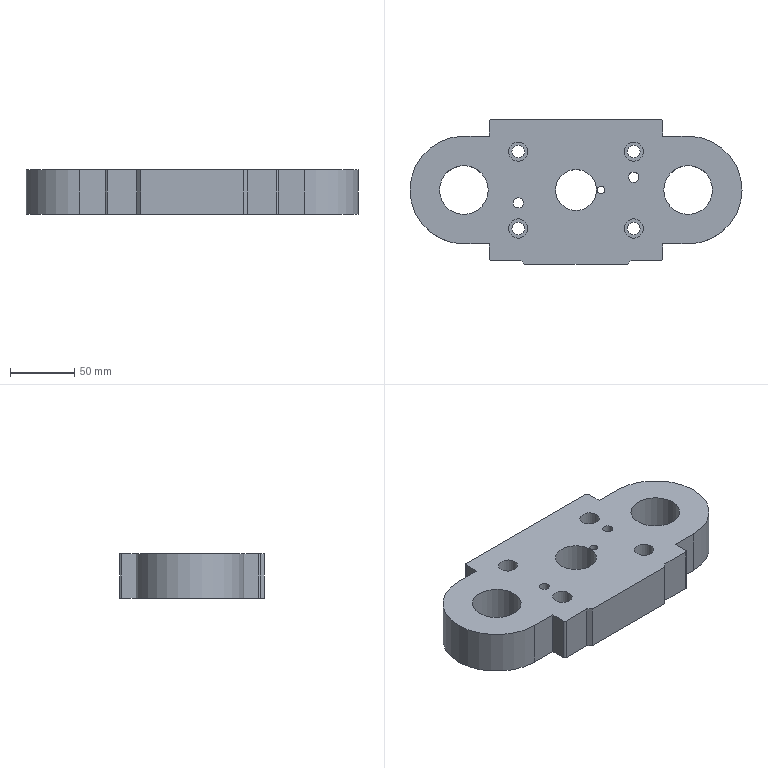Part | NX | features EXTRUDE 3, DATUM_CSYS 2, SKETCH 1 | 1 solid | 42 faces | box 259 x 113 x 35 mm | volume 709332 mm3 | cylinder 21 | plane 21 | commonest cylinder face diameters 3 x4 10 x4 15 x4 8 x2 38 x2 84 x2
STEP:
#1=CARTESIAN_POINT('',(22.5,0.,35.));
#2=VERTEX_POINT('',#1);
#3=CARTESIAN_POINT('',(19.5,0.,35.));
#4=DIRECTION('',(0.,0.,1.));
#5=DIRECTION('',(1.,0.,0.));
#6=AXIS2_PLACEMENT_3D('',#3,#4,#5);
#7=CIRCLE('',#6,3.);
#8=EDGE_CURVE('',#2,#2,#7,.T.);
#9=ORIENTED_EDGE('',*,*,#8,.T.);
#10=EDGE_LOOP('',(#9));
#11=FACE_BOUND('',#10,.T.);
#12=CARTESIAN_POINT('',(20.295,2.893,5.));
#13=VERTEX_POINT('',#12);
#14=CARTESIAN_POINT('',(20.295,-2.893,5.));
#15=VERTEX_POINT('',#14);
#16=CARTESIAN_POINT('',(19.5,0.,5.));
#17=DIRECTION('',(0.,0.,1.));
#18=DIRECTION('',(1.,0.,0.));
#19=AXIS2_PLACEMENT_3D('',#16,#17,#18);
#20=CIRCLE('',#19,3.);
#21=EDGE_CURVE('',#13,#15,#20,.T.);
#22=ORIENTED_EDGE('',*,*,#21,.F.);
#23=CARTESIAN_POINT('',(20.295,2.893,0.));
#24=VERTEX_POINT('',#23);
#25=CARTESIAN_POINT('',(20.295,2.893,2.5));
#26=DIRECTION('',(0.,0.,-1.));
#27=VECTOR('',#26,1000.);
#28=LINE('',#25,#27);
#29=EDGE_CURVE('',#13,#24,#28,.T.);
#30=ORIENTED_EDGE('',*,*,#29,.T.);
#31=CARTESIAN_POINT('',(20.295,-2.893,0.));
#32=VERTEX_POINT('',#31);
#33=CARTESIAN_POINT('',(19.5,0.,0.));
#34=DIRECTION('',(0.,0.,1.));
#35=DIRECTION('',(1.,0.,0.));
#36=AXIS2_PLACEMENT_3D('',#33,#34,#35);
#37=CIRCLE('',#36,3.);
#38=EDGE_CURVE('',#32,#24,#37,.T.);
#39=ORIENTED_EDGE('',*,*,#38,.F.);
#40=CARTESIAN_POINT('',(20.295,-2.893,2.5));
#41=DIRECTION('',(0.,0.,-1.));
#42=VECTOR('',#41,1000.);
#43=LINE('',#40,#42);
#44=EDGE_CURVE('',#32,#15,#43,.F.);
#45=ORIENTED_EDGE('',*,*,#44,.T.);
#46=EDGE_LOOP('',(#22,#30,#39,#45));
#47=FACE_BOUND('',#46,.T.);
#48=CARTESIAN_POINT('',(19.5,0.,35.));
#49=DIRECTION('',(0.,0.,-1.));
#50=DIRECTION('',(-1.,0.,0.));
#51=AXIS2_PLACEMENT_3D('',#48,#49,#50);
#52=CYLINDRICAL_SURFACE('',#51,3.);
#53=ADVANCED_FACE('',(#11,#47),#52,.F.);
#54=CARTESIAN_POINT('',(-68.5,0.,0.));
#55=VERTEX_POINT('',#54);
#56=CARTESIAN_POINT('',(-87.5,0.,0.));
#57=DIRECTION('',(0.,0.,1.));
#58=DIRECTION('',(1.,0.,0.));
#59=AXIS2_PLACEMENT_3D('',#56,#57,#58);
#60=CIRCLE('',#59,19.);
#61=EDGE_CURVE('',#55,#55,#60,.T.);
#62=ORIENTED_EDGE('',*,*,#61,.T.);
#63=EDGE_LOOP('',(#62));
#64=FACE_BOUND('',#63,.T.);
#65=CARTESIAN_POINT('',(-40.,-30.,0.));
#66=VERTEX_POINT('',#65);
#67=CARTESIAN_POINT('',(-45.,-30.,0.));
#68=DIRECTION('',(0.,0.,1.));
#69=DIRECTION('',(1.,0.,0.));
#70=AXIS2_PLACEMENT_3D('',#67,#68,#69);
#71=CIRCLE('',#70,5.);
#72=EDGE_CURVE('',#66,#66,#71,.T.);
#73=ORIENTED_EDGE('',*,*,#72,.T.);
#74=EDGE_LOOP('',(#73));
#75=FACE_BOUND('',#74,.T.);
#76=CARTESIAN_POINT('',(-40.,30.,0.));
#77=VERTEX_POINT('',#76);
#78=CARTESIAN_POINT('',(-45.,30.,0.));
#79=DIRECTION('',(0.,0.,1.));
#80=DIRECTION('',(1.,0.,0.));
#81=AXIS2_PLACEMENT_3D('',#78,#79,#80);
#82=CIRCLE('',#81,5.);
#83=EDGE_CURVE('',#77,#77,#82,.T.);
#84=ORIENTED_EDGE('',*,*,#83,.T.);
#85=EDGE_LOOP('',(#84));
#86=FACE_BOUND('',#85,.T.);
#87=CARTESIAN_POINT('',(-41.,-10.,0.));
#88=VERTEX_POINT('',#87);
#89=CARTESIAN_POINT('',(-45.,-10.,0.));
#90=DIRECTION('',(0.,0.,1.));
#91=DIRECTION('',(1.,0.,0.));
#92=AXIS2_PLACEMENT_3D('',#89,#90,#91);
#93=CIRCLE('',#92,4.);
#94=EDGE_CURVE('',#88,#88,#93,.T.);
#95=ORIENTED_EDGE('',*,*,#94,.T.);
#96=EDGE_LOOP('',(#95));
#97=FACE_BOUND('',#96,.T.);
#98=CARTESIAN_POINT('',(50.,-30.,0.));
#99=VERTEX_POINT('',#98);
#100=CARTESIAN_POINT('',(45.,-30.,0.));
#101=DIRECTION('',(0.,0.,1.));
#102=DIRECTION('',(1.,0.,0.));
#103=AXIS2_PLACEMENT_3D('',#100,#101,#102);
#104=CIRCLE('',#103,5.);
#105=EDGE_CURVE('',#99,#99,#104,.T.);
#106=ORIENTED_EDGE('',*,*,#105,.T.);
#107=EDGE_LOOP('',(#106));
#108=FACE_BOUND('',#107,.T.);
#109=CARTESIAN_POINT('',(50.,30.,0.));
#110=VERTEX_POINT('',#109);
#111=CARTESIAN_POINT('',(45.,30.,0.));
#112=DIRECTION('',(0.,0.,1.));
#113=DIRECTION('',(1.,0.,0.));
#114=AXIS2_PLACEMENT_3D('',#111,#112,#113);
#115=CIRCLE('',#114,5.);
#116=EDGE_CURVE('',#110,#110,#115,.T.);
#117=ORIENTED_EDGE('',*,*,#116,.T.);
#118=EDGE_LOOP('',(#117));
#119=FACE_BOUND('',#118,.T.);
#120=CARTESIAN_POINT('',(49.,10.,0.));
#121=VERTEX_POINT('',#120);
#122=CARTESIAN_POINT('',(45.,10.,0.));
#123=DIRECTION('',(0.,0.,1.));
#124=DIRECTION('',(1.,0.,0.));
#125=AXIS2_PLACEMENT_3D('',#122,#123,#124);
#126=CIRCLE('',#125,4.);
#127=EDGE_CURVE('',#121,#121,#126,.T.);
#128=ORIENTED_EDGE('',*,*,#127,.T.);
#129=EDGE_LOOP('',(#128));
#130=FACE_BOUND('',#129,.T.);
#131=CARTESIAN_POINT('',(106.5,0.,0.));
#132=VERTEX_POINT('',#131);
#133=CARTESIAN_POINT('',(87.5,0.,0.));
#134=DIRECTION('',(0.,0.,1.));
#135=DIRECTION('',(1.,0.,0.));
#136=AXIS2_PLACEMENT_3D('',#133,#134,#135);
#137=CIRCLE('',#136,19.);
#138=EDGE_CURVE('',#132,#132,#137,.T.);
#139=ORIENTED_EDGE('',*,*,#138,.T.);
#140=EDGE_LOOP('',(#139));
#141=FACE_BOUND('',#140,.T.);
#142=CARTESIAN_POINT('',(67.5,-42.,0.));
#143=VERTEX_POINT('',#142);
#144=CARTESIAN_POINT('',(67.5,-53.5,0.));
#145=VERTEX_POINT('',#144);
#146=CARTESIAN_POINT('',(67.5,-42.,0.));
#147=DIRECTION('',(0.,-1.,0.));
#148=VECTOR('',#147,1000.);
#149=LINE('',#146,#148);
#150=EDGE_CURVE('',#143,#145,#149,.T.);
#151=ORIENTED_EDGE('',*,*,#150,.T.);
#152=CARTESIAN_POINT('',(66.,-55.,0.));
#153=VERTEX_POINT('',#152);
#154=CARTESIAN_POINT('',(66.,-53.5,0.));
#155=DIRECTION('',(0.,0.,-1.));
#156=DIRECTION('',(1.,0.,0.));
#157=AXIS2_PLACEMENT_3D('',#154,#155,#156);
#158=CIRCLE('',#157,1.5);
#159=EDGE_CURVE('',#145,#153,#158,.T.);
#160=ORIENTED_EDGE('',*,*,#159,.T.);
#161=CARTESIAN_POINT('',(43.,-55.,0.));
#162=VERTEX_POINT('',#161);
#163=CARTESIAN_POINT('',(66.,-55.,0.));
#164=DIRECTION('',(-1.,0.,0.));
#165=VECTOR('',#164,1000.);
#166=LINE('',#163,#165);
#167=EDGE_CURVE('',#153,#162,#166,.T.);
#168=ORIENTED_EDGE('',*,*,#167,.T.);
#169=CARTESIAN_POINT('',(40.,-58.,0.));
#170=VERTEX_POINT('',#169);
#171=CARTESIAN_POINT('',(43.,-55.,0.));
#172=DIRECTION('',(-0.7071,-0.7071,0.));
#173=VECTOR('',#172,1000.);
#174=LINE('',#171,#173);
#175=EDGE_CURVE('',#162,#170,#174,.T.);
#176=ORIENTED_EDGE('',*,*,#175,.T.);
#177=CARTESIAN_POINT('',(-40.,-58.,0.));
#178=VERTEX_POINT('',#177);
#179=CARTESIAN_POINT('',(40.,-58.,0.));
#180=DIRECTION('',(-1.,0.,0.));
#181=VECTOR('',#180,1000.);
#182=LINE('',#179,#181);
#183=EDGE_CURVE('',#170,#178,#182,.T.);
#184=ORIENTED_EDGE('',*,*,#183,.T.);
#185=CARTESIAN_POINT('',(-43.,-55.,0.));
#186=VERTEX_POINT('',#185);
#187=CARTESIAN_POINT('',(-40.,-58.,0.));
#188=DIRECTION('',(-0.7071,0.7071,0.));
#189=VECTOR('',#188,1000.);
#190=LINE('',#187,#189);
#191=EDGE_CURVE('',#178,#186,#190,.T.);
#192=ORIENTED_EDGE('',*,*,#191,.T.);
#193=CARTESIAN_POINT('',(-66.,-55.,0.));
#194=VERTEX_POINT('',#193);
#195=CARTESIAN_POINT('',(-43.,-55.,0.));
#196=DIRECTION('',(-1.,0.,0.));
#197=VECTOR('',#196,1000.);
#198=LINE('',#195,#197);
#199=EDGE_CURVE('',#186,#194,#198,.T.);
#200=ORIENTED_EDGE('',*,*,#199,.T.);
#201=CARTESIAN_POINT('',(-67.5,-53.5,0.));
#202=VERTEX_POINT('',#201);
#203=CARTESIAN_POINT('',(-66.,-53.5,0.));
#204=DIRECTION('',(0.,0.,-1.));
#205=DIRECTION('',(1.,0.,0.));
#206=AXIS2_PLACEMENT_3D('',#203,#204,#205);
#207=CIRCLE('',#206,1.5);
#208=EDGE_CURVE('',#194,#202,#207,.T.);
#209=ORIENTED_EDGE('',*,*,#208,.T.);
#210=CARTESIAN_POINT('',(-67.5,-42.,0.));
#211=VERTEX_POINT('',#210);
#212=CARTESIAN_POINT('',(-67.5,-53.5,0.));
#213=DIRECTION('',(0.,1.,0.));
#214=VECTOR('',#213,1000.);
#215=LINE('',#212,#214);
#216=EDGE_CURVE('',#202,#211,#215,.T.);
#217=ORIENTED_EDGE('',*,*,#216,.T.);
#218=CARTESIAN_POINT('',(-87.5,-42.,0.));
#219=VERTEX_POINT('',#218);
#220=CARTESIAN_POINT('',(-67.5,-42.,0.));
#221=DIRECTION('',(-1.,0.,0.));
#222=VECTOR('',#221,1000.);
#223=LINE('',#220,#222);
#224=EDGE_CURVE('',#211,#219,#223,.T.);
#225=ORIENTED_EDGE('',*,*,#224,.T.);
#226=CARTESIAN_POINT('',(-87.5,42.,0.));
#227=VERTEX_POINT('',#226);
#228=CARTESIAN_POINT('',(-87.5,0.,0.));
#229=DIRECTION('',(0.,0.,-1.));
#230=DIRECTION('',(1.,0.,0.));
#231=AXIS2_PLACEMENT_3D('',#228,#229,#230);
#232=CIRCLE('',#231,42.);
#233=EDGE_CURVE('',#219,#227,#232,.T.);
#234=ORIENTED_EDGE('',*,*,#233,.T.);
#235=CARTESIAN_POINT('',(-67.5,42.,0.));
#236=VERTEX_POINT('',#235);
#237=CARTESIAN_POINT('',(-87.5,42.,0.));
#238=DIRECTION('',(1.,0.,0.));
#239=VECTOR('',#238,1000.);
#240=LINE('',#237,#239);
#241=EDGE_CURVE('',#227,#236,#240,.T.);
#242=ORIENTED_EDGE('',*,*,#241,.T.);
#243=CARTESIAN_POINT('',(-67.5,53.5,0.));
#244=VERTEX_POINT('',#243);
#245=CARTESIAN_POINT('',(-67.5,42.,0.));
#246=DIRECTION('',(0.,1.,0.));
#247=VECTOR('',#246,1000.);
#248=LINE('',#245,#247);
#249=EDGE_CURVE('',#236,#244,#248,.T.);
#250=ORIENTED_EDGE('',*,*,#249,.T.);
#251=CARTESIAN_POINT('',(-66.,55.,0.));
#252=VERTEX_POINT('',#251);
#253=CARTESIAN_POINT('',(-66.,53.5,0.));
#254=DIRECTION('',(0.,0.,-1.));
#255=DIRECTION('',(1.,0.,0.));
#256=AXIS2_PLACEMENT_3D('',#253,#254,#255);
#257=CIRCLE('',#256,1.5);
#258=EDGE_CURVE('',#244,#252,#257,.T.);
#259=ORIENTED_EDGE('',*,*,#258,.T.);
#260=CARTESIAN_POINT('',(66.,55.,0.));
#261=VERTEX_POINT('',#260);
#262=CARTESIAN_POINT('',(-66.,55.,0.));
#263=DIRECTION('',(1.,0.,0.));
#264=VECTOR('',#263,1000.);
#265=LINE('',#262,#264);
#266=EDGE_CURVE('',#252,#261,#265,.T.);
#267=ORIENTED_EDGE('',*,*,#266,.T.);
#268=CARTESIAN_POINT('',(67.5,53.5,0.));
#269=VERTEX_POINT('',#268);
#270=CARTESIAN_POINT('',(66.,53.5,0.));
#271=DIRECTION('',(0.,0.,-1.));
#272=DIRECTION('',(1.,0.,0.));
#273=AXIS2_PLACEMENT_3D('',#270,#271,#272);
#274=CIRCLE('',#273,1.5);
#275=EDGE_CURVE('',#261,#269,#274,.T.);
#276=ORIENTED_EDGE('',*,*,#275,.T.);
#277=CARTESIAN_POINT('',(67.5,42.,0.));
#278=VERTEX_POINT('',#277);
#279=CARTESIAN_POINT('',(67.5,53.5,0.));
#280=DIRECTION('',(0.,-1.,0.));
#281=VECTOR('',#280,1000.);
#282=LINE('',#279,#281);
#283=EDGE_CURVE('',#269,#278,#282,.T.);
#284=ORIENTED_EDGE('',*,*,#283,.T.);
#285=CARTESIAN_POINT('',(87.5,42.,0.));
#286=VERTEX_POINT('',#285);
#287=CARTESIAN_POINT('',(67.5,42.,0.));
#288=DIRECTION('',(1.,0.,0.));
#289=VECTOR('',#288,1000.);
#290=LINE('',#287,#289);
#291=EDGE_CURVE('',#278,#286,#290,.T.);
#292=ORIENTED_EDGE('',*,*,#291,.T.);
#293=CARTESIAN_POINT('',(87.5,-42.,0.));
#294=VERTEX_POINT('',#293);
#295=CARTESIAN_POINT('',(87.5,0.,0.));
#296=DIRECTION('',(0.,0.,-1.));
#297=DIRECTION('',(1.,0.,0.));
#298=AXIS2_PLACEMENT_3D('',#295,#296,#297);
#299=CIRCLE('',#298,42.);
#300=EDGE_CURVE('',#286,#294,#299,.T.);
#301=ORIENTED_EDGE('',*,*,#300,.T.);
#302=CARTESIAN_POINT('',(87.5,-42.,0.));
#303=DIRECTION('',(-1.,0.,0.));
#304=VECTOR('',#303,1000.);
#305=LINE('',#302,#304);
#306=EDGE_CURVE('',#294,#143,#305,.T.);
#307=ORIENTED_EDGE('',*,*,#306,.T.);
#308=EDGE_LOOP('',(#151,#160,#168,#176,#184,#192,#200,#209,#217,#225,#234,#242,#250,#259,#267,#276,#284,#292,#301,#307));
#309=FACE_BOUND('',#308,.T.);
#310=ORIENTED_EDGE('',*,*,#38,.T.);
#311=CARTESIAN_POINT('',(0.,0.,0.));
#312=DIRECTION('',(0.,0.,1.));
#313=DIRECTION('',(1.,0.,0.));
#314=AXIS2_PLACEMENT_3D('',#311,#312,#313);
#315=CIRCLE('',#314,20.5);
#316=EDGE_CURVE('',#24,#32,#315,.T.);
#317=ORIENTED_EDGE('',*,*,#316,.T.);
#318=EDGE_LOOP('',(#310,#317));
#319=FACE_BOUND('',#318,.T.);
#320=CARTESIAN_POINT('',(66.,-53.5,0.));
#321=DIRECTION('',(0.,0.,-1.));
#322=DIRECTION('',(-1.,0.,0.));
#323=AXIS2_PLACEMENT_3D('',#320,#321,#322);
#324=PLANE('',#323);
#325=ADVANCED_FACE('',(#64,#75,#86,#97,#108,#119,#130,#141,#309,#319),#324,.T.);
#326=CARTESIAN_POINT('',(-37.5,30.,35.));
#327=VERTEX_POINT('',#326);
#328=CARTESIAN_POINT('',(-45.,30.,35.));
#329=DIRECTION('',(0.,0.,1.));
#330=DIRECTION('',(1.,0.,0.));
#331=AXIS2_PLACEMENT_3D('',#328,#329,#330);
#332=CIRCLE('',#331,7.5);
#333=EDGE_CURVE('',#327,#327,#332,.T.);
#334=ORIENTED_EDGE('',*,*,#333,.F.);
#335=EDGE_LOOP('',(#334));
#336=FACE_BOUND('',#335,.T.);
#337=CARTESIAN_POINT('',(52.5,30.,35.));
#338=VERTEX_POINT('',#337);
#339=CARTESIAN_POINT('',(45.,30.,35.));
#340=DIRECTION('',(0.,0.,1.));
#341=DIRECTION('',(1.,0.,0.));
#342=AXIS2_PLACEMENT_3D('',#339,#340,#341);
#343=CIRCLE('',#342,7.5);
#344=EDGE_CURVE('',#338,#338,#343,.T.);
#345=ORIENTED_EDGE('',*,*,#344,.F.);
#346=EDGE_LOOP('',(#345));
#347=FACE_BOUND('',#346,.T.);
#348=CARTESIAN_POINT('',(67.5,-42.,35.));
#349=VERTEX_POINT('',#348);
#350=CARTESIAN_POINT('',(67.5,-53.5,35.));
#351=VERTEX_POINT('',#350);
#352=CARTESIAN_POINT('',(67.5,-42.,35.));
#353=DIRECTION('',(0.,-1.,0.));
#354=VECTOR('',#353,1000.);
#355=LINE('',#352,#354);
#356=EDGE_CURVE('',#349,#351,#355,.T.);
#357=ORIENTED_EDGE('',*,*,#356,.F.);
#358=CARTESIAN_POINT('',(87.5,-42.,35.));
#359=VERTEX_POINT('',#358);
#360=CARTESIAN_POINT('',(87.5,-42.,35.));
#361=DIRECTION('',(-1.,0.,0.));
#362=VECTOR('',#361,1000.);
#363=LINE('',#360,#362);
#364=EDGE_CURVE('',#359,#349,#363,.T.);
#365=ORIENTED_EDGE('',*,*,#364,.F.);
#366=CARTESIAN_POINT('',(87.5,42.,35.));
#367=VERTEX_POINT('',#366);
#368=CARTESIAN_POINT('',(87.5,0.,35.));
#369=DIRECTION('',(0.,0.,-1.));
#370=DIRECTION('',(1.,0.,0.));
#371=AXIS2_PLACEMENT_3D('',#368,#369,#370);
#372=CIRCLE('',#371,42.);
#373=EDGE_CURVE('',#367,#359,#372,.T.);
#374=ORIENTED_EDGE('',*,*,#373,.F.);
#375=CARTESIAN_POINT('',(67.5,42.,35.));
#376=VERTEX_POINT('',#375);
#377=CARTESIAN_POINT('',(67.5,42.,35.));
#378=DIRECTION('',(1.,0.,0.));
#379=VECTOR('',#378,1000.);
#380=LINE('',#377,#379);
#381=EDGE_CURVE('',#376,#367,#380,.T.);
#382=ORIENTED_EDGE('',*,*,#381,.F.);
#383=CARTESIAN_POINT('',(67.5,53.5,35.));
#384=VERTEX_POINT('',#383);
#385=CARTESIAN_POINT('',(67.5,53.5,35.));
#386=DIRECTION('',(0.,-1.,0.));
#387=VECTOR('',#386,1000.);
#388=LINE('',#385,#387);
#389=EDGE_CURVE('',#384,#376,#388,.T.);
#390=ORIENTED_EDGE('',*,*,#389,.F.);
#391=CARTESIAN_POINT('',(66.,55.,35.));
#392=VERTEX_POINT('',#391);
#393=CARTESIAN_POINT('',(66.,53.5,35.));
#394=DIRECTION('',(0.,0.,-1.));
#395=DIRECTION('',(1.,0.,0.));
#396=AXIS2_PLACEMENT_3D('',#393,#394,#395);
#397=CIRCLE('',#396,1.5);
#398=EDGE_CURVE('',#392,#384,#397,.T.);
#399=ORIENTED_EDGE('',*,*,#398,.F.);
#400=CARTESIAN_POINT('',(-66.,55.,35.));
#401=VERTEX_POINT('',#400);
#402=CARTESIAN_POINT('',(-66.,55.,35.));
#403=DIRECTION('',(1.,0.,0.));
#404=VECTOR('',#403,1000.);
#405=LINE('',#402,#404);
#406=EDGE_CURVE('',#401,#392,#405,.T.);
#407=ORIENTED_EDGE('',*,*,#406,.F.);
#408=CARTESIAN_POINT('',(-67.5,53.5,35.));
#409=VERTEX_POINT('',#408);
#410=CARTESIAN_POINT('',(-66.,53.5,35.));
#411=DIRECTION('',(0.,0.,-1.));
#412=DIRECTION('',(1.,0.,0.));
#413=AXIS2_PLACEMENT_3D('',#410,#411,#412);
#414=CIRCLE('',#413,1.5);
#415=EDGE_CURVE('',#409,#401,#414,.T.);
#416=ORIENTED_EDGE('',*,*,#415,.F.);
#417=CARTESIAN_POINT('',(-67.5,42.,35.));
#418=VERTEX_POINT('',#417);
#419=CARTESIAN_POINT('',(-67.5,42.,35.));
#420=DIRECTION('',(0.,1.,0.));
#421=VECTOR('',#420,1000.);
#422=LINE('',#419,#421);
#423=EDGE_CURVE('',#418,#409,#422,.T.);
#424=ORIENTED_EDGE('',*,*,#423,.F.);
#425=CARTESIAN_POINT('',(-87.5,42.,35.));
#426=VERTEX_POINT('',#425);
#427=CARTESIAN_POINT('',(-87.5,42.,35.));
#428=DIRECTION('',(1.,0.,0.));
#429=VECTOR('',#428,1000.);
#430=LINE('',#427,#429);
#431=EDGE_CURVE('',#426,#418,#430,.T.);
#432=ORIENTED_EDGE('',*,*,#431,.F.);
#433=CARTESIAN_POINT('',(-87.5,-42.,35.));
#434=VERTEX_POINT('',#433);
#435=CARTESIAN_POINT('',(-87.5,0.,35.));
#436=DIRECTION('',(0.,0.,-1.));
#437=DIRECTION('',(1.,0.,0.));
#438=AXIS2_PLACEMENT_3D('',#435,#436,#437);
#439=CIRCLE('',#438,42.);
#440=EDGE_CURVE('',#434,#426,#439,.T.);
#441=ORIENTED_EDGE('',*,*,#440,.F.);
#442=CARTESIAN_POINT('',(-67.5,-42.,35.));
#443=VERTEX_POINT('',#442);
#444=CARTESIAN_POINT('',(-67.5,-42.,35.));
#445=DIRECTION('',(-1.,0.,0.));
#446=VECTOR('',#445,1000.);
#447=LINE('',#444,#446);
#448=EDGE_CURVE('',#443,#434,#447,.T.);
#449=ORIENTED_EDGE('',*,*,#448,.F.);
#450=CARTESIAN_POINT('',(-67.5,-53.5,35.));
#451=VERTEX_POINT('',#450);
#452=CARTESIAN_POINT('',(-67.5,-53.5,35.));
#453=DIRECTION('',(0.,1.,0.));
#454=VECTOR('',#453,1000.);
#455=LINE('',#452,#454);
#456=EDGE_CURVE('',#451,#443,#455,.T.);
#457=ORIENTED_EDGE('',*,*,#456,.F.);
#458=CARTESIAN_POINT('',(-66.,-55.,35.));
#459=VERTEX_POINT('',#458);
#460=CARTESIAN_POINT('',(-66.,-53.5,35.));
#461=DIRECTION('',(0.,0.,-1.));
#462=DIRECTION('',(1.,0.,0.));
#463=AXIS2_PLACEMENT_3D('',#460,#461,#462);
#464=CIRCLE('',#463,1.5);
#465=EDGE_CURVE('',#459,#451,#464,.T.);
#466=ORIENTED_EDGE('',*,*,#465,.F.);
#467=CARTESIAN_POINT('',(-43.,-55.,35.));
#468=VERTEX_POINT('',#467);
#469=CARTESIAN_POINT('',(-43.,-55.,35.));
#470=DIRECTION('',(-1.,0.,0.));
#471=VECTOR('',#470,1000.);
#472=LINE('',#469,#471);
#473=EDGE_CURVE('',#468,#459,#472,.T.);
#474=ORIENTED_EDGE('',*,*,#473,.F.);
#475=CARTESIAN_POINT('',(-40.,-58.,35.));
#476=VERTEX_POINT('',#475);
#477=CARTESIAN_POINT('',(-40.,-58.,35.));
#478=DIRECTION('',(-0.7071,0.7071,0.));
#479=VECTOR('',#478,1000.);
#480=LINE('',#477,#479);
#481=EDGE_CURVE('',#476,#468,#480,.T.);
#482=ORIENTED_EDGE('',*,*,#481,.F.);
#483=CARTESIAN_POINT('',(40.,-58.,35.));
#484=VERTEX_POINT('',#483);
#485=CARTESIAN_POINT('',(40.,-58.,35.));
#486=DIRECTION('',(-1.,0.,0.));
#487=VECTOR('',#486,1000.);
#488=LINE('',#485,#487);
#489=EDGE_CURVE('',#484,#476,#488,.T.);
#490=ORIENTED_EDGE('',*,*,#489,.F.);
#491=CARTESIAN_POINT('',(43.,-55.,35.));
#492=VERTEX_POINT('',#491);
#493=CARTESIAN_POINT('',(43.,-55.,35.));
#494=DIRECTION('',(-0.7071,-0.7071,0.));
#495=VECTOR('',#494,1000.);
#496=LINE('',#493,#495);
#497=EDGE_CURVE('',#492,#484,#496,.T.);
#498=ORIENTED_EDGE('',*,*,#497,.F.);
#499=CARTESIAN_POINT('',(66.,-55.,35.));
#500=VERTEX_POINT('',#499);
#501=CARTESIAN_POINT('',(66.,-55.,35.));
#502=DIRECTION('',(-1.,0.,0.));
#503=VECTOR('',#502,1000.);
#504=LINE('',#501,#503);
#505=EDGE_CURVE('',#500,#492,#504,.T.);
#506=ORIENTED_EDGE('',*,*,#505,.F.);
#507=CARTESIAN_POINT('',(66.,-53.5,35.));
#508=DIRECTION('',(0.,0.,-1.));
#509=DIRECTION('',(1.,0.,0.));
#510=AXIS2_PLACEMENT_3D('',#507,#508,#509);
#511=CIRCLE('',#510,1.5);
#512=EDGE_CURVE('',#351,#500,#511,.T.);
#513=ORIENTED_EDGE('',*,*,#512,.F.);
#514=EDGE_LOOP('',(#357,#365,#374,#382,#390,#399,#407,#416,#424,#432,#441,#449,#457,#466,#474,#482,#490,#498,#506,#513));
#515=FACE_BOUND('',#514,.T.);
#516=CARTESIAN_POINT('',(106.5,0.,35.));
#517=VERTEX_POINT('',#516);
#518=CARTESIAN_POINT('',(87.5,0.,35.));
#519=DIRECTION('',(0.,0.,1.));
#520=DIRECTION('',(1.,0.,0.));
#521=AXIS2_PLACEMENT_3D('',#518,#519,#520);
#522=CIRCLE('',#521,19.);
#523=EDGE_CURVE('',#517,#517,#522,.T.);
#524=ORIENTED_EDGE('',*,*,#523,.F.);
#525=EDGE_LOOP('',(#524));
#526=FACE_BOUND('',#525,.T.);
#527=CARTESIAN_POINT('',(49.,10.,35.));
#528=VERTEX_POINT('',#527);
#529=CARTESIAN_POINT('',(45.,10.,35.));
#530=DIRECTION('',(0.,0.,1.));
#531=DIRECTION('',(1.,0.,0.));
#532=AXIS2_PLACEMENT_3D('',#529,#530,#531);
#533=CIRCLE('',#532,4.);
#534=EDGE_CURVE('',#528,#528,#533,.T.);
#535=ORIENTED_EDGE('',*,*,#534,.F.);
#536=EDGE_LOOP('',(#535));
#537=FACE_BOUND('',#536,.T.);
#538=ORIENTED_EDGE('',*,*,#8,.F.);
#539=EDGE_LOOP('',(#538));
#540=FACE_BOUND('',#539,.T.);
#541=CARTESIAN_POINT('',(16.,0.,35.));
#542=VERTEX_POINT('',#541);
#543=CARTESIAN_POINT('',(0.,0.,35.));
#544=DIRECTION('',(0.,0.,1.));
#545=DIRECTION('',(1.,0.,0.));
#546=AXIS2_PLACEMENT_3D('',#543,#544,#545);
#547=CIRCLE('',#546,16.);
#548=EDGE_CURVE('',#542,#542,#547,.T.);
#549=ORIENTED_EDGE('',*,*,#548,.F.);
#550=EDGE_LOOP('',(#549));
#551=FACE_BOUND('',#550,.T.);
#552=CARTESIAN_POINT('',(-41.,-10.,35.));
#553=VERTEX_POINT('',#552);
#554=CARTESIAN_POINT('',(-45.,-10.,35.));
#555=DIRECTION('',(0.,0.,1.));
#556=DIRECTION('',(1.,0.,0.));
#557=AXIS2_PLACEMENT_3D('',#554,#555,#556);
#558=CIRCLE('',#557,4.);
#559=EDGE_CURVE('',#553,#553,#558,.T.);
#560=ORIENTED_EDGE('',*,*,#559,.F.);
#561=EDGE_LOOP('',(#560));
#562=FACE_BOUND('',#561,.T.);
#563=CARTESIAN_POINT('',(-68.5,0.,35.));
#564=VERTEX_POINT('',#563);
#565=CARTESIAN_POINT('',(-87.5,0.,35.));
#566=DIRECTION('',(0.,0.,1.));
#567=DIRECTION('',(1.,0.,0.));
#568=AXIS2_PLACEMENT_3D('',#565,#566,#567);
#569=CIRCLE('',#568,19.);
#570=EDGE_CURVE('',#564,#564,#569,.T.);
#571=ORIENTED_EDGE('',*,*,#570,.F.);
#572=EDGE_LOOP('',(#571));
#573=FACE_BOUND('',#572,.T.);
#574=CARTESIAN_POINT('',(52.5,-30.,35.));
#575=VERTEX_POINT('',#574);
#576=CARTESIAN_POINT('',(45.,-30.,35.));
#577=DIRECTION('',(0.,0.,1.));
#578=DIRECTION('',(1.,0.,0.));
#579=AXIS2_PLACEMENT_3D('',#576,#577,#578);
#580=CIRCLE('',#579,7.5);
#581=EDGE_CURVE('',#575,#575,#580,.T.);
#582=ORIENTED_EDGE('',*,*,#581,.F.);
#583=EDGE_LOOP('',(#582));
#584=FACE_BOUND('',#583,.T.);
#585=CARTESIAN_POINT('',(-37.5,-30.,35.));
#586=VERTEX_POINT('',#585);
#587=CARTESIAN_POINT('',(-45.,-30.,35.));
#588=DIRECTION('',(0.,0.,1.));
#589=DIRECTION('',(1.,0.,0.));
#590=AXIS2_PLACEMENT_3D('',#587,#588,#589);
#591=CIRCLE('',#590,7.5);
#592=EDGE_CURVE('',#586,#586,#591,.T.);
#593=ORIENTED_EDGE('',*,*,#592,.F.);
#594=EDGE_LOOP('',(#593));
#595=FACE_BOUND('',#594,.T.);
#596=CARTESIAN_POINT('',(66.,-53.5,35.));
#597=DIRECTION('',(0.,0.,-1.));
#598=DIRECTION('',(-1.,0.,0.));
#599=AXIS2_PLACEMENT_3D('',#596,#597,#598);
#600=PLANE('',#599);
#601=ADVANCED_FACE('',(#336,#347,#515,#526,#537,#540,#551,#562,#573,#584,#595),#600,.F.);
#602=ORIENTED_EDGE('',*,*,#72,.F.);
#603=EDGE_LOOP('',(#602));
#604=FACE_BOUND('',#603,.T.);
#605=CARTESIAN_POINT('',(-40.,-30.,22.));
#606=VERTEX_POINT('',#605);
#607=CARTESIAN_POINT('',(-45.,-30.,22.));
#608=DIRECTION('',(0.,0.,1.));
#609=DIRECTION('',(1.,0.,0.));
#610=AXIS2_PLACEMENT_3D('',#607,#608,#609);
#611=CIRCLE('',#610,5.);
#612=EDGE_CURVE('',#606,#606,#611,.T.);
#613=ORIENTED_EDGE('',*,*,#612,.T.);
#614=EDGE_LOOP('',(#613));
#615=FACE_BOUND('',#614,.T.);
#616=CARTESIAN_POINT('',(-45.,-30.,35.));
#617=DIRECTION('',(0.,0.,-1.));
#618=DIRECTION('',(-1.,0.,0.));
#619=AXIS2_PLACEMENT_3D('',#616,#617,#618);
#620=CYLINDRICAL_SURFACE('',#619,5.);
#621=ADVANCED_FACE('',(#604,#615),#620,.F.);
#622=ORIENTED_EDGE('',*,*,#83,.F.);
#623=EDGE_LOOP('',(#622));
#624=FACE_BOUND('',#623,.T.);
#625=CARTESIAN_POINT('',(-40.,30.,22.));
#626=VERTEX_POINT('',#625);
#627=CARTESIAN_POINT('',(-45.,30.,22.));
#628=DIRECTION('',(0.,0.,1.));
#629=DIRECTION('',(1.,0.,0.));
#630=AXIS2_PLACEMENT_3D('',#627,#628,#629);
#631=CIRCLE('',#630,5.);
#632=EDGE_CURVE('',#626,#626,#631,.T.);
#633=ORIENTED_EDGE('',*,*,#632,.T.);
#634=EDGE_LOOP('',(#633));
#635=FACE_BOUND('',#634,.T.);
#636=CARTESIAN_POINT('',(-45.,30.,35.));
#637=DIRECTION('',(0.,0.,-1.));
#638=DIRECTION('',(-1.,0.,0.));
#639=AXIS2_PLACEMENT_3D('',#636,#637,#638);
#640=CYLINDRICAL_SURFACE('',#639,5.);
#641=ADVANCED_FACE('',(#624,#635),#640,.F.);
#642=ORIENTED_EDGE('',*,*,#105,.F.);
#643=EDGE_LOOP('',(#642));
#644=FACE_BOUND('',#643,.T.);
#645=CARTESIAN_POINT('',(50.,-30.,22.));
#646=VERTEX_POINT('',#645);
#647=CARTESIAN_POINT('',(45.,-30.,22.));
#648=DIRECTION('',(0.,0.,1.));
#649=DIRECTION('',(1.,0.,0.));
#650=AXIS2_PLACEMENT_3D('',#647,#648,#649);
#651=CIRCLE('',#650,5.);
#652=EDGE_CURVE('',#646,#646,#651,.T.);
#653=ORIENTED_EDGE('',*,*,#652,.T.);
#654=EDGE_LOOP('',(#653));
#655=FACE_BOUND('',#654,.T.);
#656=CARTESIAN_POINT('',(45.,-30.,35.));
#657=DIRECTION('',(0.,0.,-1.));
#658=DIRECTION('',(-1.,0.,0.));
#659=AXIS2_PLACEMENT_3D('',#656,#657,#658);
#660=CYLINDRICAL_SURFACE('',#659,5.);
#661=ADVANCED_FACE('',(#644,#655),#660,.F.);
#662=ORIENTED_EDGE('',*,*,#116,.F.);
#663=EDGE_LOOP('',(#662));
#664=FACE_BOUND('',#663,.T.);
#665=CARTESIAN_POINT('',(50.,30.,22.));
#666=VERTEX_POINT('',#665);
#667=CARTESIAN_POINT('',(45.,30.,22.));
#668=DIRECTION('',(0.,0.,1.));
#669=DIRECTION('',(1.,0.,0.));
#670=AXIS2_PLACEMENT_3D('',#667,#668,#669);
#671=CIRCLE('',#670,5.);
#672=EDGE_CURVE('',#666,#666,#671,.T.);
#673=ORIENTED_EDGE('',*,*,#672,.T.);
#674=EDGE_LOOP('',(#673));
#675=FACE_BOUND('',#674,.T.);
#676=CARTESIAN_POINT('',(45.,30.,35.));
#677=DIRECTION('',(0.,0.,-1.));
#678=DIRECTION('',(-1.,0.,0.));
#679=AXIS2_PLACEMENT_3D('',#676,#677,#678);
#680=CYLINDRICAL_SURFACE('',#679,5.);
#681=ADVANCED_FACE('',(#664,#675),#680,.F.);
#682=ORIENTED_EDGE('',*,*,#150,.F.);
#683=CARTESIAN_POINT('',(67.5,-42.,35.));
#684=DIRECTION('',(0.,0.,-1.));
#685=VECTOR('',#684,1000.);
#686=LINE('',#683,#685);
#687=EDGE_CURVE('',#349,#143,#686,.T.);
#688=ORIENTED_EDGE('',*,*,#687,.F.);
#689=ORIENTED_EDGE('',*,*,#356,.T.);
#690=CARTESIAN_POINT('',(67.5,-53.5,35.));
#691=DIRECTION('',(0.,0.,-1.));
#692=VECTOR('',#691,1000.);
#693=LINE('',#690,#692);
#694=EDGE_CURVE('',#351,#145,#693,.T.);
#695=ORIENTED_EDGE('',*,*,#694,.T.);
#696=EDGE_LOOP('',(#682,#688,#689,#695));
#697=FACE_BOUND('',#696,.T.);
#698=CARTESIAN_POINT('',(67.5,-42.,35.));
#699=DIRECTION('',(1.,0.,0.));
#700=DIRECTION('',(0.,0.,-1.));
#701=AXIS2_PLACEMENT_3D('',#698,#699,#700);
#702=PLANE('',#701);
#703=ADVANCED_FACE('',(#697),#702,.T.);
#704=ORIENTED_EDGE('',*,*,#159,.F.);
#705=ORIENTED_EDGE('',*,*,#694,.F.);
#706=ORIENTED_EDGE('',*,*,#512,.T.);
#707=CARTESIAN_POINT('',(66.,-55.,35.));
#708=DIRECTION('',(0.,0.,-1.));
#709=VECTOR('',#708,1000.);
#710=LINE('',#707,#709);
#711=EDGE_CURVE('',#500,#153,#710,.T.);
#712=ORIENTED_EDGE('',*,*,#711,.T.);
#713=EDGE_LOOP('',(#704,#705,#706,#712));
#714=FACE_BOUND('',#713,.T.);
#715=CARTESIAN_POINT('',(66.,-53.5,35.));
#716=DIRECTION('',(0.,0.,-1.));
#717=DIRECTION('',(-1.,0.,0.));
#718=AXIS2_PLACEMENT_3D('',#715,#716,#717);
#719=CYLINDRICAL_SURFACE('',#718,1.5);
#720=ADVANCED_FACE('',(#714),#719,.T.);
#721=ORIENTED_EDGE('',*,*,#167,.F.);
#722=ORIENTED_EDGE('',*,*,#711,.F.);
#723=ORIENTED_EDGE('',*,*,#505,.T.);
#724=CARTESIAN_POINT('',(43.,-55.,35.));
#725=DIRECTION('',(0.,0.,-1.));
#726=VECTOR('',#725,1000.);
#727=LINE('',#724,#726);
#728=EDGE_CURVE('',#492,#162,#727,.T.);
#729=ORIENTED_EDGE('',*,*,#728,.T.);
#730=EDGE_LOOP('',(#721,#722,#723,#729));
#731=FACE_BOUND('',#730,.T.);
#732=CARTESIAN_POINT('',(66.,-55.,35.));
#733=DIRECTION('',(0.,-1.,0.));
#734=DIRECTION('',(0.,0.,-1.));
#735=AXIS2_PLACEMENT_3D('',#732,#733,#734);
#736=PLANE('',#735);
#737=ADVANCED_FACE('',(#731),#736,.T.);
#738=ORIENTED_EDGE('',*,*,#175,.F.);
#739=ORIENTED_EDGE('',*,*,#728,.F.);
#740=ORIENTED_EDGE('',*,*,#497,.T.);
#741=CARTESIAN_POINT('',(40.,-58.,35.));
#742=DIRECTION('',(0.,0.,-1.));
#743=VECTOR('',#742,1000.);
#744=LINE('',#741,#743);
#745=EDGE_CURVE('',#484,#170,#744,.T.);
#746=ORIENTED_EDGE('',*,*,#745,.T.);
#747=EDGE_LOOP('',(#738,#739,#740,#746));
#748=FACE_BOUND('',#747,.T.);
#749=CARTESIAN_POINT('',(43.,-55.,35.));
#750=DIRECTION('',(0.7071,-0.7071,0.));
#751=DIRECTION('',(0.7071,0.7071,0.));
#752=AXIS2_PLACEMENT_3D('',#749,#750,#751);
#753=PLANE('',#752);
#754=ADVANCED_FACE('',(#748),#753,.T.);
#755=ORIENTED_EDGE('',*,*,#183,.F.);
#756=ORIENTED_EDGE('',*,*,#745,.F.);
#757=ORIENTED_EDGE('',*,*,#489,.T.);
#758=CARTESIAN_POINT('',(-40.,-58.,35.));
#759=DIRECTION('',(0.,0.,-1.));
#760=VECTOR('',#759,1000.);
#761=LINE('',#758,#760);
#762=EDGE_CURVE('',#476,#178,#761,.T.);
#763=ORIENTED_EDGE('',*,*,#762,.T.);
#764=EDGE_LOOP('',(#755,#756,#757,#763));
#765=FACE_BOUND('',#764,.T.);
#766=CARTESIAN_POINT('',(40.,-58.,35.));
#767=DIRECTION('',(0.,-1.,0.));
#768=DIRECTION('',(0.,0.,-1.));
#769=AXIS2_PLACEMENT_3D('',#766,#767,#768);
#770=PLANE('',#769);
#771=ADVANCED_FACE('',(#765),#770,.T.);
#772=ORIENTED_EDGE('',*,*,#191,.F.);
#773=ORIENTED_EDGE('',*,*,#762,.F.);
#774=ORIENTED_EDGE('',*,*,#481,.T.);
#775=CARTESIAN_POINT('',(-43.,-55.,35.));
#776=DIRECTION('',(0.,0.,-1.));
#777=VECTOR('',#776,1000.);
#778=LINE('',#775,#777);
#779=EDGE_CURVE('',#468,#186,#778,.T.);
#780=ORIENTED_EDGE('',*,*,#779,.T.);
#781=EDGE_LOOP('',(#772,#773,#774,#780));
#782=FACE_BOUND('',#781,.T.);
#783=CARTESIAN_POINT('',(-40.,-58.,35.));
#784=DIRECTION('',(-0.7071,-0.7071,0.));
#785=DIRECTION('',(0.7071,-0.7071,0.));
#786=AXIS2_PLACEMENT_3D('',#783,#784,#785);
#787=PLANE('',#786);
#788=ADVANCED_FACE('',(#782),#787,.T.);
#789=ORIENTED_EDGE('',*,*,#199,.F.);
#790=ORIENTED_EDGE('',*,*,#779,.F.);
#791=ORIENTED_EDGE('',*,*,#473,.T.);
#792=CARTESIAN_POINT('',(-66.,-55.,35.));
#793=DIRECTION('',(0.,0.,-1.));
#794=VECTOR('',#793,1000.);
#795=LINE('',#792,#794);
#796=EDGE_CURVE('',#459,#194,#795,.T.);
#797=ORIENTED_EDGE('',*,*,#796,.T.);
#798=EDGE_LOOP('',(#789,#790,#791,#797));
#799=FACE_BOUND('',#798,.T.);
#800=CARTESIAN_POINT('',(-43.,-55.,35.));
#801=DIRECTION('',(0.,-1.,0.));
#802=DIRECTION('',(0.,0.,-1.));
#803=AXIS2_PLACEMENT_3D('',#800,#801,#802);
#804=PLANE('',#803);
#805=ADVANCED_FACE('',(#799),#804,.T.);
#806=ORIENTED_EDGE('',*,*,#208,.F.);
#807=ORIENTED_EDGE('',*,*,#796,.F.);
#808=ORIENTED_EDGE('',*,*,#465,.T.);
#809=CARTESIAN_POINT('',(-67.5,-53.5,35.));
#810=DIRECTION('',(0.,0.,-1.));
#811=VECTOR('',#810,1000.);
#812=LINE('',#809,#811);
#813=EDGE_CURVE('',#451,#202,#812,.T.);
#814=ORIENTED_EDGE('',*,*,#813,.T.);
#815=EDGE_LOOP('',(#806,#807,#808,#814));
#816=FACE_BOUND('',#815,.T.);
#817=CARTESIAN_POINT('',(-66.,-53.5,35.));
#818=DIRECTION('',(0.,0.,-1.));
#819=DIRECTION('',(-1.,0.,0.));
#820=AXIS2_PLACEMENT_3D('',#817,#818,#819);
#821=CYLINDRICAL_SURFACE('',#820,1.5);
#822=ADVANCED_FACE('',(#816),#821,.T.);
#823=ORIENTED_EDGE('',*,*,#216,.F.);
#824=ORIENTED_EDGE('',*,*,#813,.F.);
#825=ORIENTED_EDGE('',*,*,#456,.T.);
#826=CARTESIAN_POINT('',(-67.5,-42.,35.));
#827=DIRECTION('',(0.,0.,-1.));
#828=VECTOR('',#827,1000.);
#829=LINE('',#826,#828);
#830=EDGE_CURVE('',#443,#211,#829,.T.);
#831=ORIENTED_EDGE('',*,*,#830,.T.);
#832=EDGE_LOOP('',(#823,#824,#825,#831));
#833=FACE_BOUND('',#832,.T.);
#834=CARTESIAN_POINT('',(-67.5,-53.5,35.));
#835=DIRECTION('',(-1.,0.,0.));
#836=DIRECTION('',(0.,0.,1.));
#837=AXIS2_PLACEMENT_3D('',#834,#835,#836);
#838=PLANE('',#837);
#839=ADVANCED_FACE('',(#833),#838,.T.);
#840=ORIENTED_EDGE('',*,*,#224,.F.);
#841=ORIENTED_EDGE('',*,*,#830,.F.);
#842=ORIENTED_EDGE('',*,*,#448,.T.);
#843=CARTESIAN_POINT('',(-87.5,-42.,35.));
#844=DIRECTION('',(0.,0.,-1.));
#845=VECTOR('',#844,1000.);
#846=LINE('',#843,#845);
#847=EDGE_CURVE('',#434,#219,#846,.T.);
#848=ORIENTED_EDGE('',*,*,#847,.T.);
#849=EDGE_LOOP('',(#840,#841,#842,#848));
#850=FACE_BOUND('',#849,.T.);
#851=CARTESIAN_POINT('',(-67.5,-42.,35.));
#852=DIRECTION('',(0.,-1.,0.));
#853=DIRECTION('',(0.,0.,-1.));
#854=AXIS2_PLACEMENT_3D('',#851,#852,#853);
#855=PLANE('',#854);
#856=ADVANCED_FACE('',(#850),#855,.T.);
#857=ORIENTED_EDGE('',*,*,#233,.F.);
#858=ORIENTED_EDGE('',*,*,#847,.F.);
#859=ORIENTED_EDGE('',*,*,#440,.T.);
#860=CARTESIAN_POINT('',(-87.5,42.,35.));
#861=DIRECTION('',(0.,0.,-1.));
#862=VECTOR('',#861,1000.);
#863=LINE('',#860,#862);
#864=EDGE_CURVE('',#426,#227,#863,.T.);
#865=ORIENTED_EDGE('',*,*,#864,.T.);
#866=EDGE_LOOP('',(#857,#858,#859,#865));
#867=FACE_BOUND('',#866,.T.);
#868=CARTESIAN_POINT('',(-87.5,0.,35.));
#869=DIRECTION('',(0.,0.,-1.));
#870=DIRECTION('',(-1.,0.,0.));
#871=AXIS2_PLACEMENT_3D('',#868,#869,#870);
#872=CYLINDRICAL_SURFACE('',#871,42.);
#873=ADVANCED_FACE('',(#867),#872,.T.);
#874=ORIENTED_EDGE('',*,*,#241,.F.);
#875=ORIENTED_EDGE('',*,*,#864,.F.);
#876=ORIENTED_EDGE('',*,*,#431,.T.);
#877=CARTESIAN_POINT('',(-67.5,42.,35.));
#878=DIRECTION('',(0.,0.,-1.));
#879=VECTOR('',#878,1000.);
#880=LINE('',#877,#879);
#881=EDGE_CURVE('',#418,#236,#880,.T.);
#882=ORIENTED_EDGE('',*,*,#881,.T.);
#883=EDGE_LOOP('',(#874,#875,#876,#882));
#884=FACE_BOUND('',#883,.T.);
#885=CARTESIAN_POINT('',(-87.5,42.,35.));
#886=DIRECTION('',(0.,1.,0.));
#887=DIRECTION('',(0.,0.,1.));
#888=AXIS2_PLACEMENT_3D('',#885,#886,#887);
#889=PLANE('',#888);
#890=ADVANCED_FACE('',(#884),#889,.T.);
#891=ORIENTED_EDGE('',*,*,#249,.F.);
#892=ORIENTED_EDGE('',*,*,#881,.F.);
#893=ORIENTED_EDGE('',*,*,#423,.T.);
#894=CARTESIAN_POINT('',(-67.5,53.5,35.));
#895=DIRECTION('',(0.,0.,-1.));
#896=VECTOR('',#895,1000.);
#897=LINE('',#894,#896);
#898=EDGE_CURVE('',#409,#244,#897,.T.);
#899=ORIENTED_EDGE('',*,*,#898,.T.);
#900=EDGE_LOOP('',(#891,#892,#893,#899));
#901=FACE_BOUND('',#900,.T.);
#902=CARTESIAN_POINT('',(-67.5,42.,35.));
#903=DIRECTION('',(-1.,0.,0.));
#904=DIRECTION('',(0.,0.,1.));
#905=AXIS2_PLACEMENT_3D('',#902,#903,#904);
#906=PLANE('',#905);
#907=ADVANCED_FACE('',(#901),#906,.T.);
#908=ORIENTED_EDGE('',*,*,#258,.F.);
#909=ORIENTED_EDGE('',*,*,#898,.F.);
#910=ORIENTED_EDGE('',*,*,#415,.T.);
#911=CARTESIAN_POINT('',(-66.,55.,35.));
#912=DIRECTION('',(0.,0.,-1.));
#913=VECTOR('',#912,1000.);
#914=LINE('',#911,#913);
#915=EDGE_CURVE('',#401,#252,#914,.T.);
#916=ORIENTED_EDGE('',*,*,#915,.T.);
#917=EDGE_LOOP('',(#908,#909,#910,#916));
#918=FACE_BOUND('',#917,.T.);
#919=CARTESIAN_POINT('',(-66.,53.5,35.));
#920=DIRECTION('',(0.,0.,-1.));
#921=DIRECTION('',(-1.,0.,0.));
#922=AXIS2_PLACEMENT_3D('',#919,#920,#921);
#923=CYLINDRICAL_SURFACE('',#922,1.5);
#924=ADVANCED_FACE('',(#918),#923,.T.);
#925=ORIENTED_EDGE('',*,*,#266,.F.);
#926=ORIENTED_EDGE('',*,*,#915,.F.);
#927=ORIENTED_EDGE('',*,*,#406,.T.);
#928=CARTESIAN_POINT('',(66.,55.,35.));
#929=DIRECTION('',(0.,0.,-1.));
#930=VECTOR('',#929,1000.);
#931=LINE('',#928,#930);
#932=EDGE_CURVE('',#392,#261,#931,.T.);
#933=ORIENTED_EDGE('',*,*,#932,.T.);
#934=EDGE_LOOP('',(#925,#926,#927,#933));
#935=FACE_BOUND('',#934,.T.);
#936=CARTESIAN_POINT('',(-66.,55.,35.));
#937=DIRECTION('',(0.,1.,0.));
#938=DIRECTION('',(0.,0.,1.));
#939=AXIS2_PLACEMENT_3D('',#936,#937,#938);
#940=PLANE('',#939);
#941=ADVANCED_FACE('',(#935),#940,.T.);
#942=ORIENTED_EDGE('',*,*,#275,.F.);
#943=ORIENTED_EDGE('',*,*,#932,.F.);
#944=ORIENTED_EDGE('',*,*,#398,.T.);
#945=CARTESIAN_POINT('',(67.5,53.5,35.));
#946=DIRECTION('',(0.,0.,-1.));
#947=VECTOR('',#946,1000.);
#948=LINE('',#945,#947);
#949=EDGE_CURVE('',#384,#269,#948,.T.);
#950=ORIENTED_EDGE('',*,*,#949,.T.);
#951=EDGE_LOOP('',(#942,#943,#944,#950));
#952=FACE_BOUND('',#951,.T.);
#953=CARTESIAN_POINT('',(66.,53.5,35.));
#954=DIRECTION('',(0.,0.,-1.));
#955=DIRECTION('',(-1.,0.,0.));
#956=AXIS2_PLACEMENT_3D('',#953,#954,#955);
#957=CYLINDRICAL_SURFACE('',#956,1.5);
#958=ADVANCED_FACE('',(#952),#957,.T.);
#959=ORIENTED_EDGE('',*,*,#283,.F.);
#960=ORIENTED_EDGE('',*,*,#949,.F.);
#961=ORIENTED_EDGE('',*,*,#389,.T.);
#962=CARTESIAN_POINT('',(67.5,42.,35.));
#963=DIRECTION('',(0.,0.,-1.));
#964=VECTOR('',#963,1000.);
#965=LINE('',#962,#964);
#966=EDGE_CURVE('',#376,#278,#965,.T.);
#967=ORIENTED_EDGE('',*,*,#966,.T.);
#968=EDGE_LOOP('',(#959,#960,#961,#967));
#969=FACE_BOUND('',#968,.T.);
#970=CARTESIAN_POINT('',(67.5,53.5,35.));
#971=DIRECTION('',(1.,0.,0.));
#972=DIRECTION('',(0.,0.,-1.));
#973=AXIS2_PLACEMENT_3D('',#970,#971,#972);
#974=PLANE('',#973);
#975=ADVANCED_FACE('',(#969),#974,.T.);
#976=ORIENTED_EDGE('',*,*,#291,.F.);
#977=ORIENTED_EDGE('',*,*,#966,.F.);
#978=ORIENTED_EDGE('',*,*,#381,.T.);
#979=CARTESIAN_POINT('',(87.5,42.,35.));
#980=DIRECTION('',(0.,0.,-1.));
#981=VECTOR('',#980,1000.);
#982=LINE('',#979,#981);
#983=EDGE_CURVE('',#367,#286,#982,.T.);
#984=ORIENTED_EDGE('',*,*,#983,.T.);
#985=EDGE_LOOP('',(#976,#977,#978,#984));
#986=FACE_BOUND('',#985,.T.);
#987=CARTESIAN_POINT('',(67.5,42.,35.));
#988=DIRECTION('',(0.,1.,0.));
#989=DIRECTION('',(0.,0.,1.));
#990=AXIS2_PLACEMENT_3D('',#987,#988,#989);
#991=PLANE('',#990);
#992=ADVANCED_FACE('',(#986),#991,.T.);
#993=ORIENTED_EDGE('',*,*,#300,.F.);
#994=ORIENTED_EDGE('',*,*,#983,.F.);
#995=ORIENTED_EDGE('',*,*,#373,.T.);
#996=CARTESIAN_POINT('',(87.5,-42.,35.));
#997=DIRECTION('',(0.,0.,-1.));
#998=VECTOR('',#997,1000.);
#999=LINE('',#996,#998);
#1000=EDGE_CURVE('',#359,#294,#999,.T.);
#1001=ORIENTED_EDGE('',*,*,#1000,.T.);
#1002=EDGE_LOOP('',(#993,#994,#995,#1001));
#1003=FACE_BOUND('',#1002,.T.);
#1004=CARTESIAN_POINT('',(87.5,0.,35.));
#1005=DIRECTION('',(0.,0.,-1.));
#1006=DIRECTION('',(-1.,0.,0.));
#1007=AXIS2_PLACEMENT_3D('',#1004,#1005,#1006);
#1008=CYLINDRICAL_SURFACE('',#1007,42.);
#1009=ADVANCED_FACE('',(#1003),#1008,.T.);
#1010=ORIENTED_EDGE('',*,*,#559,.T.);
#1011=EDGE_LOOP('',(#1010));
#1012=FACE_BOUND('',#1011,.T.);
#1013=ORIENTED_EDGE('',*,*,#94,.F.);
#1014=EDGE_LOOP('',(#1013));
#1015=FACE_BOUND('',#1014,.T.);
#1016=CARTESIAN_POINT('',(-45.,-10.,35.));
#1017=DIRECTION('',(0.,0.,-1.));
#1018=DIRECTION('',(-1.,0.,0.));
#1019=AXIS2_PLACEMENT_3D('',#1016,#1017,#1018);
#1020=CYLINDRICAL_SURFACE('',#1019,4.);
#1021=ADVANCED_FACE('',(#1012,#1015),#1020,.F.);
#1022=CARTESIAN_POINT('',(16.,0.,5.));
#1023=VERTEX_POINT('',#1022);
#1024=CARTESIAN_POINT('',(0.,0.,5.));
#1025=DIRECTION('',(0.,0.,1.));
#1026=DIRECTION('',(1.,0.,0.));
#1027=AXIS2_PLACEMENT_3D('',#1024,#1025,#1026);
#1028=CIRCLE('',#1027,16.);
#1029=EDGE_CURVE('',#1023,#1023,#1028,.T.);
#1030=ORIENTED_EDGE('',*,*,#1029,.F.);
#1031=EDGE_LOOP('',(#1030));
#1032=FACE_BOUND('',#1031,.T.);
#1033=ORIENTED_EDGE('',*,*,#548,.T.);
#1034=EDGE_LOOP('',(#1033));
#1035=FACE_BOUND('',#1034,.T.);
#1036=CARTESIAN_POINT('',(0.,0.,35.));
#1037=DIRECTION('',(0.,0.,-1.));
#1038=DIRECTION('',(-1.,0.,0.));
#1039=AXIS2_PLACEMENT_3D('',#1036,#1037,#1038);
#1040=CYLINDRICAL_SURFACE('',#1039,16.);
#1041=ADVANCED_FACE('',(#1032,#1035),#1040,.F.);
#1042=ORIENTED_EDGE('',*,*,#534,.T.);
#1043=EDGE_LOOP('',(#1042));
#1044=FACE_BOUND('',#1043,.T.);
#1045=ORIENTED_EDGE('',*,*,#127,.F.);
#1046=EDGE_LOOP('',(#1045));
#1047=FACE_BOUND('',#1046,.T.);
#1048=CARTESIAN_POINT('',(45.,10.,35.));
#1049=DIRECTION('',(0.,0.,-1.));
#1050=DIRECTION('',(-1.,0.,0.));
#1051=AXIS2_PLACEMENT_3D('',#1048,#1049,#1050);
#1052=CYLINDRICAL_SURFACE('',#1051,4.);
#1053=ADVANCED_FACE('',(#1044,#1047),#1052,.F.);
#1054=ORIENTED_EDGE('',*,*,#523,.T.);
#1055=EDGE_LOOP('',(#1054));
#1056=FACE_BOUND('',#1055,.T.);
#1057=ORIENTED_EDGE('',*,*,#138,.F.);
#1058=EDGE_LOOP('',(#1057));
#1059=FACE_BOUND('',#1058,.T.);
#1060=CARTESIAN_POINT('',(87.5,0.,35.));
#1061=DIRECTION('',(0.,0.,-1.));
#1062=DIRECTION('',(-1.,0.,0.));
#1063=AXIS2_PLACEMENT_3D('',#1060,#1061,#1062);
#1064=CYLINDRICAL_SURFACE('',#1063,19.);
#1065=ADVANCED_FACE('',(#1056,#1059),#1064,.F.);
#1066=ORIENTED_EDGE('',*,*,#306,.F.);
#1067=ORIENTED_EDGE('',*,*,#1000,.F.);
#1068=ORIENTED_EDGE('',*,*,#364,.T.);
#1069=ORIENTED_EDGE('',*,*,#687,.T.);
#1070=EDGE_LOOP('',(#1066,#1067,#1068,#1069));
#1071=FACE_BOUND('',#1070,.T.);
#1072=CARTESIAN_POINT('',(87.5,-42.,35.));
#1073=DIRECTION('',(0.,-1.,0.));
#1074=DIRECTION('',(0.,0.,-1.));
#1075=AXIS2_PLACEMENT_3D('',#1072,#1073,#1074);
#1076=PLANE('',#1075);
#1077=ADVANCED_FACE('',(#1071),#1076,.T.);
#1078=ORIENTED_EDGE('',*,*,#570,.T.);
#1079=EDGE_LOOP('',(#1078));
#1080=FACE_BOUND('',#1079,.T.);
#1081=ORIENTED_EDGE('',*,*,#61,.F.);
#1082=EDGE_LOOP('',(#1081));
#1083=FACE_BOUND('',#1082,.T.);
#1084=CARTESIAN_POINT('',(-87.5,0.,35.));
#1085=DIRECTION('',(0.,0.,-1.));
#1086=DIRECTION('',(-1.,0.,0.));
#1087=AXIS2_PLACEMENT_3D('',#1084,#1085,#1086);
#1088=CYLINDRICAL_SURFACE('',#1087,19.);
#1089=ADVANCED_FACE('',(#1080,#1083),#1088,.F.);
#1090=ORIENTED_EDGE('',*,*,#344,.T.);
#1091=EDGE_LOOP('',(#1090));
#1092=FACE_BOUND('',#1091,.T.);
#1093=CARTESIAN_POINT('',(52.5,30.,22.));
#1094=VERTEX_POINT('',#1093);
#1095=CARTESIAN_POINT('',(45.,30.,22.));
#1096=DIRECTION('',(0.,0.,1.));
#1097=DIRECTION('',(1.,0.,0.));
#1098=AXIS2_PLACEMENT_3D('',#1095,#1096,#1097);
#1099=CIRCLE('',#1098,7.5);
#1100=EDGE_CURVE('',#1094,#1094,#1099,.F.);
#1101=ORIENTED_EDGE('',*,*,#1100,.T.);
#1102=EDGE_LOOP('',(#1101));
#1103=FACE_BOUND('',#1102,.T.);
#1104=CARTESIAN_POINT('',(45.,30.,35.));
#1105=DIRECTION('',(0.,0.,-1.));
#1106=DIRECTION('',(-1.,0.,0.));
#1107=AXIS2_PLACEMENT_3D('',#1104,#1105,#1106);
#1108=CYLINDRICAL_SURFACE('',#1107,7.5);
#1109=ADVANCED_FACE('',(#1092,#1103),#1108,.F.);
#1110=ORIENTED_EDGE('',*,*,#672,.F.);
#1111=EDGE_LOOP('',(#1110));
#1112=FACE_BOUND('',#1111,.T.);
#1113=ORIENTED_EDGE('',*,*,#1100,.F.);
#1114=EDGE_LOOP('',(#1113));
#1115=FACE_BOUND('',#1114,.T.);
#1116=CARTESIAN_POINT('',(45.,30.,22.));
#1117=DIRECTION('',(0.,0.,1.));
#1118=DIRECTION('',(1.,0.,0.));
#1119=AXIS2_PLACEMENT_3D('',#1116,#1117,#1118);
#1120=PLANE('',#1119);
#1121=ADVANCED_FACE('',(#1112,#1115),#1120,.T.);
#1122=ORIENTED_EDGE('',*,*,#581,.T.);
#1123=EDGE_LOOP('',(#1122));
#1124=FACE_BOUND('',#1123,.T.);
#1125=CARTESIAN_POINT('',(52.5,-30.,22.));
#1126=VERTEX_POINT('',#1125);
#1127=CARTESIAN_POINT('',(45.,-30.,22.));
#1128=DIRECTION('',(0.,0.,1.));
#1129=DIRECTION('',(1.,0.,0.));
#1130=AXIS2_PLACEMENT_3D('',#1127,#1128,#1129);
#1131=CIRCLE('',#1130,7.5);
#1132=EDGE_CURVE('',#1126,#1126,#1131,.F.);
#1133=ORIENTED_EDGE('',*,*,#1132,.T.);
#1134=EDGE_LOOP('',(#1133));
#1135=FACE_BOUND('',#1134,.T.);
#1136=CARTESIAN_POINT('',(45.,-30.,35.));
#1137=DIRECTION('',(0.,0.,-1.));
#1138=DIRECTION('',(-1.,0.,0.));
#1139=AXIS2_PLACEMENT_3D('',#1136,#1137,#1138);
#1140=CYLINDRICAL_SURFACE('',#1139,7.5);
#1141=ADVANCED_FACE('',(#1124,#1135),#1140,.F.);
#1142=ORIENTED_EDGE('',*,*,#652,.F.);
#1143=EDGE_LOOP('',(#1142));
#1144=FACE_BOUND('',#1143,.T.);
#1145=ORIENTED_EDGE('',*,*,#1132,.F.);
#1146=EDGE_LOOP('',(#1145));
#1147=FACE_BOUND('',#1146,.T.);
#1148=CARTESIAN_POINT('',(45.,-30.,22.));
#1149=DIRECTION('',(0.,0.,1.));
#1150=DIRECTION('',(1.,0.,0.));
#1151=AXIS2_PLACEMENT_3D('',#1148,#1149,#1150);
#1152=PLANE('',#1151);
#1153=ADVANCED_FACE('',(#1144,#1147),#1152,.T.);
#1154=ORIENTED_EDGE('',*,*,#333,.T.);
#1155=EDGE_LOOP('',(#1154));
#1156=FACE_BOUND('',#1155,.T.);
#1157=CARTESIAN_POINT('',(-37.5,30.,22.));
#1158=VERTEX_POINT('',#1157);
#1159=CARTESIAN_POINT('',(-45.,30.,22.));
#1160=DIRECTION('',(0.,0.,1.));
#1161=DIRECTION('',(1.,0.,0.));
#1162=AXIS2_PLACEMENT_3D('',#1159,#1160,#1161);
#1163=CIRCLE('',#1162,7.5);
#1164=EDGE_CURVE('',#1158,#1158,#1163,.F.);
#1165=ORIENTED_EDGE('',*,*,#1164,.T.);
#1166=EDGE_LOOP('',(#1165));
#1167=FACE_BOUND('',#1166,.T.);
#1168=CARTESIAN_POINT('',(-45.,30.,35.));
#1169=DIRECTION('',(0.,0.,-1.));
#1170=DIRECTION('',(-1.,0.,0.));
#1171=AXIS2_PLACEMENT_3D('',#1168,#1169,#1170);
#1172=CYLINDRICAL_SURFACE('',#1171,7.5);
#1173=ADVANCED_FACE('',(#1156,#1167),#1172,.F.);
#1174=ORIENTED_EDGE('',*,*,#632,.F.);
#1175=EDGE_LOOP('',(#1174));
#1176=FACE_BOUND('',#1175,.T.);
#1177=ORIENTED_EDGE('',*,*,#1164,.F.);
#1178=EDGE_LOOP('',(#1177));
#1179=FACE_BOUND('',#1178,.T.);
#1180=CARTESIAN_POINT('',(-45.,30.,22.));
#1181=DIRECTION('',(0.,0.,1.));
#1182=DIRECTION('',(1.,0.,0.));
#1183=AXIS2_PLACEMENT_3D('',#1180,#1181,#1182);
#1184=PLANE('',#1183);
#1185=ADVANCED_FACE('',(#1176,#1179),#1184,.T.);
#1186=ORIENTED_EDGE('',*,*,#592,.T.);
#1187=EDGE_LOOP('',(#1186));
#1188=FACE_BOUND('',#1187,.T.);
#1189=CARTESIAN_POINT('',(-37.5,-30.,22.));
#1190=VERTEX_POINT('',#1189);
#1191=CARTESIAN_POINT('',(-45.,-30.,22.));
#1192=DIRECTION('',(0.,0.,1.));
#1193=DIRECTION('',(1.,0.,0.));
#1194=AXIS2_PLACEMENT_3D('',#1191,#1192,#1193);
#1195=CIRCLE('',#1194,7.5);
#1196=EDGE_CURVE('',#1190,#1190,#1195,.F.);
#1197=ORIENTED_EDGE('',*,*,#1196,.T.);
#1198=EDGE_LOOP('',(#1197));
#1199=FACE_BOUND('',#1198,.T.);
#1200=CARTESIAN_POINT('',(-45.,-30.,35.));
#1201=DIRECTION('',(0.,0.,-1.));
#1202=DIRECTION('',(-1.,0.,0.));
#1203=AXIS2_PLACEMENT_3D('',#1200,#1201,#1202);
#1204=CYLINDRICAL_SURFACE('',#1203,7.5);
#1205=ADVANCED_FACE('',(#1188,#1199),#1204,.F.);
#1206=ORIENTED_EDGE('',*,*,#612,.F.);
#1207=EDGE_LOOP('',(#1206));
#1208=FACE_BOUND('',#1207,.T.);
#1209=ORIENTED_EDGE('',*,*,#1196,.F.);
#1210=EDGE_LOOP('',(#1209));
#1211=FACE_BOUND('',#1210,.T.);
#1212=CARTESIAN_POINT('',(-45.,-30.,22.));
#1213=DIRECTION('',(0.,0.,1.));
#1214=DIRECTION('',(1.,0.,0.));
#1215=AXIS2_PLACEMENT_3D('',#1212,#1213,#1214);
#1216=PLANE('',#1215);
#1217=ADVANCED_FACE('',(#1208,#1211),#1216,.T.);
#1218=CARTESIAN_POINT('',(0.,0.,5.));
#1219=DIRECTION('',(0.,0.,1.));
#1220=DIRECTION('',(1.,0.,0.));
#1221=AXIS2_PLACEMENT_3D('',#1218,#1219,#1220);
#1222=CIRCLE('',#1221,20.5);
#1223=EDGE_CURVE('',#15,#13,#1222,.F.);
#1224=ORIENTED_EDGE('',*,*,#1223,.F.);
#1225=ORIENTED_EDGE('',*,*,#44,.F.);
#1226=ORIENTED_EDGE('',*,*,#316,.F.);
#1227=ORIENTED_EDGE('',*,*,#29,.F.);
#1228=EDGE_LOOP('',(#1224,#1225,#1226,#1227));
#1229=FACE_BOUND('',#1228,.T.);
#1230=CARTESIAN_POINT('',(0.,0.,5.));
#1231=DIRECTION('',(0.,0.,-1.));
#1232=DIRECTION('',(-1.,0.,0.));
#1233=AXIS2_PLACEMENT_3D('',#1230,#1231,#1232);
#1234=CYLINDRICAL_SURFACE('',#1233,20.5);
#1235=ADVANCED_FACE('',(#1229),#1234,.F.);
#1236=ORIENTED_EDGE('',*,*,#1029,.T.);
#1237=EDGE_LOOP('',(#1236));
#1238=FACE_BOUND('',#1237,.T.);
#1239=ORIENTED_EDGE('',*,*,#21,.T.);
#1240=ORIENTED_EDGE('',*,*,#1223,.T.);
#1241=EDGE_LOOP('',(#1239,#1240));
#1242=FACE_BOUND('',#1241,.T.);
#1243=CARTESIAN_POINT('',(0.,0.,5.));
#1244=DIRECTION('',(0.,0.,1.));
#1245=DIRECTION('',(1.,0.,0.));
#1246=AXIS2_PLACEMENT_3D('',#1243,#1244,#1245);
#1247=PLANE('',#1246);
#1248=ADVANCED_FACE('',(#1238,#1242),#1247,.F.);
#1249=CLOSED_SHELL('',(#53,#325,#601,#621,#641,#661,#681,#703,#720,#737,#754,#771,#788,#805,#822,#839,#856,#873,#890,#907,#924,#941,#958,#975,#992,#1009,#1021,#1041,#1053,#1065,#1077,#1089,#1109,#1121,#1141,#1153,#1173,#1185,#1205,#1217,#1235,#1248));
#1250=MANIFOLD_SOLID_BREP('',#1249);
#1251=(LENGTH_UNIT()NAMED_UNIT(*)SI_UNIT(.MILLI.,.METRE.));
#1252=UNCERTAINTY_MEASURE_WITH_UNIT(LENGTH_MEASURE(0.00001),#1251,'','');
#1253=(NAMED_UNIT(*)PLANE_ANGLE_UNIT()SI_UNIT($,.RADIAN.));
#1254=(NAMED_UNIT(*)SI_UNIT($,.STERADIAN.)SOLID_ANGLE_UNIT());
#1255=(GEOMETRIC_REPRESENTATION_CONTEXT(3)GLOBAL_UNCERTAINTY_ASSIGNED_CONTEXT((#1252))GLOBAL_UNIT_ASSIGNED_CONTEXT((#1251,#1253,#1254))REPRESENTATION_CONTEXT('',''));
#1256=ADVANCED_BREP_SHAPE_REPRESENTATION('',(#1250),#1255);